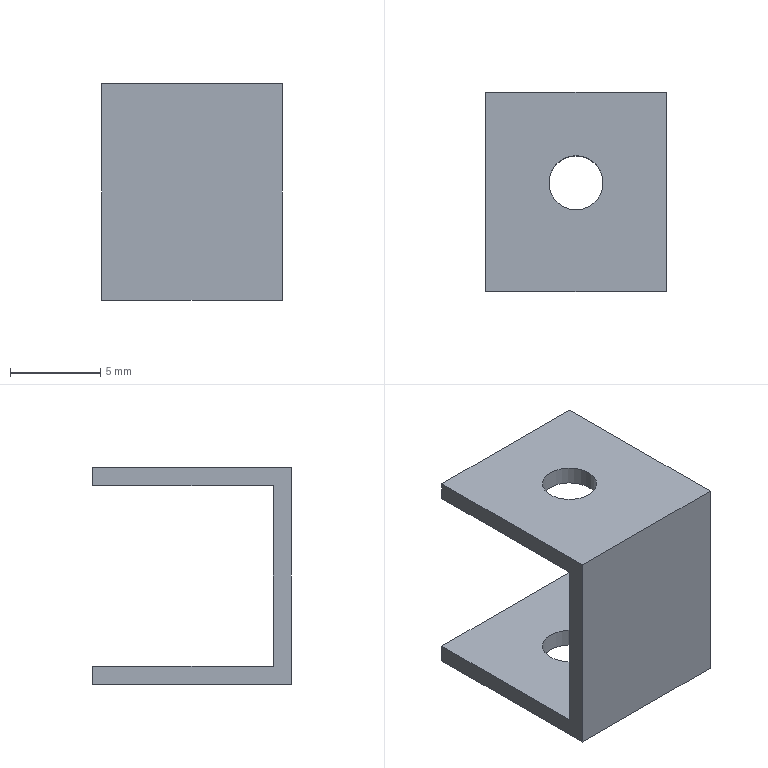Part | STEP file | 1-41.5 | 1 solid | 12 faces | box 10 x 11 x 12 mm | volume 305.863 mm3 | plane 10 | cylinder 2 | commonest cylinder face diameters 3 x2
STEP:
#1=CARTESIAN_POINT('',(0.,0.,0.));
#2=DIRECTION('',(0.,0.,1.));
#3=DIRECTION('',(1.,0.,0.));
#4=AXIS2_PLACEMENT_3D('',#1,#2,#3);
#5=CARTESIAN_POINT('',(5.,-5.5,-6.));
#6=VERTEX_POINT('',#5);
#7=CARTESIAN_POINT('',(5.,5.5,-6.));
#8=VERTEX_POINT('',#7);
#9=CARTESIAN_POINT('',(5.,-5.5,-6.));
#10=DIRECTION('',(0.,1.,0.));
#11=VECTOR('',#10,1.);
#12=LINE('',#9,#11);
#13=CARTESIAN_POINT('',(5.,0.5,0.));
#14=DIRECTION('',(1.,0.,0.));
#15=DIRECTION('',(0.,1.,0.));
#16=AXIS2_PLACEMENT_3D('',#13,#14,#15);
#17=PLANE('',#16);
#18=CARTESIAN_POINT('',(-6.,-6.));
#19=DIRECTION('',(1.,0.));
#20=VECTOR('',#19,1.);
#21=LINE('',#18,#20);
#22=(GEOMETRIC_REPRESENTATION_CONTEXT(2)PARAMETRIC_REPRESENTATION_CONTEXT()REPRESENTATION_CONTEXT('',''));
#23=DEFINITIONAL_REPRESENTATION('',(#21),#22);
#24=PCURVE('',#17,#23);
#25=CARTESIAN_POINT('',(0.,0.,-6.));
#26=DIRECTION('',(0.,0.,1.));
#27=DIRECTION('',(0.,1.,0.));
#28=AXIS2_PLACEMENT_3D('',#25,#26,#27);
#29=PLANE('',#28);
#30=CARTESIAN_POINT('',(-5.5,-5.));
#31=DIRECTION('',(1.,0.));
#32=VECTOR('',#31,1.);
#33=LINE('',#30,#32);
#34=(GEOMETRIC_REPRESENTATION_CONTEXT(2)PARAMETRIC_REPRESENTATION_CONTEXT()REPRESENTATION_CONTEXT('',''));
#35=DEFINITIONAL_REPRESENTATION('',(#33),#34);
#36=PCURVE('',#29,#35);
#37=SURFACE_CURVE('',#12,(#24,#36),.PCURVE_S1.);
#38=EDGE_CURVE('',#6,#8,#37,.T.);
#39=ORIENTED_EDGE('',*,*,#38,.T.);
#40=CARTESIAN_POINT('',(5.,5.5,-5.));
#41=VERTEX_POINT('',#40);
#42=CARTESIAN_POINT('',(5.,5.5,-6.));
#43=DIRECTION('',(0.,0.,1.));
#44=VECTOR('',#43,1.);
#45=LINE('',#42,#44);
#46=CARTESIAN_POINT('',(5.,-6.));
#47=DIRECTION('',(0.,1.));
#48=VECTOR('',#47,1.);
#49=LINE('',#46,#48);
#50=(GEOMETRIC_REPRESENTATION_CONTEXT(2)PARAMETRIC_REPRESENTATION_CONTEXT()REPRESENTATION_CONTEXT('',''));
#51=DEFINITIONAL_REPRESENTATION('',(#49),#50);
#52=PCURVE('',#17,#51);
#53=CARTESIAN_POINT('',(0.,5.5,-5.5));
#54=DIRECTION('',(0.,-1.,0.));
#55=DIRECTION('',(0.,0.,1.));
#56=AXIS2_PLACEMENT_3D('',#53,#54,#55);
#57=PLANE('',#56);
#58=CARTESIAN_POINT('',(-0.5,-5.));
#59=DIRECTION('',(1.,0.));
#60=VECTOR('',#59,1.);
#61=LINE('',#58,#60);
#62=(GEOMETRIC_REPRESENTATION_CONTEXT(2)PARAMETRIC_REPRESENTATION_CONTEXT()REPRESENTATION_CONTEXT('',''));
#63=DEFINITIONAL_REPRESENTATION('',(#61),#62);
#64=PCURVE('',#57,#63);
#65=SURFACE_CURVE('',#45,(#52,#64),.PCURVE_S1.);
#66=EDGE_CURVE('',#8,#41,#65,.T.);
#67=ORIENTED_EDGE('',*,*,#66,.T.);
#68=CARTESIAN_POINT('',(5.,-4.5,-5.));
#69=VERTEX_POINT('',#68);
#70=CARTESIAN_POINT('',(5.,5.5,-5.));
#71=DIRECTION('',(0.,-1.,0.));
#72=VECTOR('',#71,1.);
#73=LINE('',#70,#72);
#74=CARTESIAN_POINT('',(5.,-5.));
#75=DIRECTION('',(-1.,0.));
#76=VECTOR('',#75,1.);
#77=LINE('',#74,#76);
#78=(GEOMETRIC_REPRESENTATION_CONTEXT(2)PARAMETRIC_REPRESENTATION_CONTEXT()REPRESENTATION_CONTEXT('',''));
#79=DEFINITIONAL_REPRESENTATION('',(#77),#78);
#80=PCURVE('',#17,#79);
#81=CARTESIAN_POINT('',(0.,0.5,-5.));
#82=DIRECTION('',(0.,0.,-1.));
#83=DIRECTION('',(0.,-1.,0.));
#84=AXIS2_PLACEMENT_3D('',#81,#82,#83);
#85=PLANE('',#84);
#86=CARTESIAN_POINT('',(-5.,-5.));
#87=DIRECTION('',(1.,0.));
#88=VECTOR('',#87,1.);
#89=LINE('',#86,#88);
#90=(GEOMETRIC_REPRESENTATION_CONTEXT(2)PARAMETRIC_REPRESENTATION_CONTEXT()REPRESENTATION_CONTEXT('',''));
#91=DEFINITIONAL_REPRESENTATION('',(#89),#90);
#92=PCURVE('',#85,#91);
#93=SURFACE_CURVE('',#73,(#80,#92),.PCURVE_S1.);
#94=EDGE_CURVE('',#41,#69,#93,.T.);
#95=ORIENTED_EDGE('',*,*,#94,.T.);
#96=CARTESIAN_POINT('',(5.,-4.5,5.));
#97=VERTEX_POINT('',#96);
#98=CARTESIAN_POINT('',(5.,-4.5,-5.));
#99=DIRECTION('',(0.,0.,1.));
#100=VECTOR('',#99,1.);
#101=LINE('',#98,#100);
#102=CARTESIAN_POINT('',(-5.,-5.));
#103=DIRECTION('',(0.,1.));
#104=VECTOR('',#103,1.);
#105=LINE('',#102,#104);
#106=(GEOMETRIC_REPRESENTATION_CONTEXT(2)PARAMETRIC_REPRESENTATION_CONTEXT()REPRESENTATION_CONTEXT('',''));
#107=DEFINITIONAL_REPRESENTATION('',(#105),#106);
#108=PCURVE('',#17,#107);
#109=CARTESIAN_POINT('',(0.,-4.5,0.));
#110=DIRECTION('',(0.,-1.,0.));
#111=DIRECTION('',(0.,0.,1.));
#112=AXIS2_PLACEMENT_3D('',#109,#110,#111);
#113=PLANE('',#112);
#114=CARTESIAN_POINT('',(-5.,-5.));
#115=DIRECTION('',(1.,0.));
#116=VECTOR('',#115,1.);
#117=LINE('',#114,#116);
#118=(GEOMETRIC_REPRESENTATION_CONTEXT(2)PARAMETRIC_REPRESENTATION_CONTEXT()REPRESENTATION_CONTEXT('',''));
#119=DEFINITIONAL_REPRESENTATION('',(#117),#118);
#120=PCURVE('',#113,#119);
#121=SURFACE_CURVE('',#101,(#108,#120),.PCURVE_S1.);
#122=EDGE_CURVE('',#69,#97,#121,.T.);
#123=ORIENTED_EDGE('',*,*,#122,.T.);
#124=CARTESIAN_POINT('',(5.,5.5,5.));
#125=VERTEX_POINT('',#124);
#126=CARTESIAN_POINT('',(5.,-4.5,5.));
#127=DIRECTION('',(0.,1.,0.));
#128=VECTOR('',#127,1.);
#129=LINE('',#126,#128);
#130=CARTESIAN_POINT('',(-5.,5.));
#131=DIRECTION('',(1.,0.));
#132=VECTOR('',#131,1.);
#133=LINE('',#130,#132);
#134=(GEOMETRIC_REPRESENTATION_CONTEXT(2)PARAMETRIC_REPRESENTATION_CONTEXT()REPRESENTATION_CONTEXT('',''));
#135=DEFINITIONAL_REPRESENTATION('',(#133),#134);
#136=PCURVE('',#17,#135);
#137=CARTESIAN_POINT('',(0.,0.5,5.));
#138=DIRECTION('',(0.,0.,1.));
#139=DIRECTION('',(0.,1.,0.));
#140=AXIS2_PLACEMENT_3D('',#137,#138,#139);
#141=PLANE('',#140);
#142=CARTESIAN_POINT('',(-5.,-5.));
#143=DIRECTION('',(1.,0.));
#144=VECTOR('',#143,1.);
#145=LINE('',#142,#144);
#146=(GEOMETRIC_REPRESENTATION_CONTEXT(2)PARAMETRIC_REPRESENTATION_CONTEXT()REPRESENTATION_CONTEXT('',''));
#147=DEFINITIONAL_REPRESENTATION('',(#145),#146);
#148=PCURVE('',#141,#147);
#149=SURFACE_CURVE('',#129,(#136,#148),.PCURVE_S1.);
#150=EDGE_CURVE('',#97,#125,#149,.T.);
#151=ORIENTED_EDGE('',*,*,#150,.T.);
#152=CARTESIAN_POINT('',(5.,5.5,6.));
#153=VERTEX_POINT('',#152);
#154=CARTESIAN_POINT('',(5.,5.5,5.));
#155=DIRECTION('',(0.,0.,1.));
#156=VECTOR('',#155,1.);
#157=LINE('',#154,#156);
#158=CARTESIAN_POINT('',(5.,5.));
#159=DIRECTION('',(0.,1.));
#160=VECTOR('',#159,1.);
#161=LINE('',#158,#160);
#162=(GEOMETRIC_REPRESENTATION_CONTEXT(2)PARAMETRIC_REPRESENTATION_CONTEXT()REPRESENTATION_CONTEXT('',''));
#163=DEFINITIONAL_REPRESENTATION('',(#161),#162);
#164=PCURVE('',#17,#163);
#165=CARTESIAN_POINT('',(0.,5.5,5.5));
#166=DIRECTION('',(0.,-1.,0.));
#167=DIRECTION('',(0.,0.,1.));
#168=AXIS2_PLACEMENT_3D('',#165,#166,#167);
#169=PLANE('',#168);
#170=CARTESIAN_POINT('',(-0.5,-5.));
#171=DIRECTION('',(1.,0.));
#172=VECTOR('',#171,1.);
#173=LINE('',#170,#172);
#174=(GEOMETRIC_REPRESENTATION_CONTEXT(2)PARAMETRIC_REPRESENTATION_CONTEXT()REPRESENTATION_CONTEXT('',''));
#175=DEFINITIONAL_REPRESENTATION('',(#173),#174);
#176=PCURVE('',#169,#175);
#177=SURFACE_CURVE('',#157,(#164,#176),.PCURVE_S1.);
#178=EDGE_CURVE('',#125,#153,#177,.T.);
#179=ORIENTED_EDGE('',*,*,#178,.T.);
#180=CARTESIAN_POINT('',(5.,-5.5,6.));
#181=VERTEX_POINT('',#180);
#182=CARTESIAN_POINT('',(5.,5.5,6.));
#183=DIRECTION('',(0.,-1.,0.));
#184=VECTOR('',#183,1.);
#185=LINE('',#182,#184);
#186=CARTESIAN_POINT('',(5.,6.));
#187=DIRECTION('',(-1.,0.));
#188=VECTOR('',#187,1.);
#189=LINE('',#186,#188);
#190=(GEOMETRIC_REPRESENTATION_CONTEXT(2)PARAMETRIC_REPRESENTATION_CONTEXT()REPRESENTATION_CONTEXT('',''));
#191=DEFINITIONAL_REPRESENTATION('',(#189),#190);
#192=PCURVE('',#17,#191);
#193=CARTESIAN_POINT('',(0.,0.,6.));
#194=DIRECTION('',(0.,0.,-1.));
#195=DIRECTION('',(0.,-1.,0.));
#196=AXIS2_PLACEMENT_3D('',#193,#194,#195);
#197=PLANE('',#196);
#198=CARTESIAN_POINT('',(-5.5,-5.));
#199=DIRECTION('',(1.,0.));
#200=VECTOR('',#199,1.);
#201=LINE('',#198,#200);
#202=(GEOMETRIC_REPRESENTATION_CONTEXT(2)PARAMETRIC_REPRESENTATION_CONTEXT()REPRESENTATION_CONTEXT('',''));
#203=DEFINITIONAL_REPRESENTATION('',(#201),#202);
#204=PCURVE('',#197,#203);
#205=SURFACE_CURVE('',#185,(#192,#204),.PCURVE_S1.);
#206=EDGE_CURVE('',#153,#181,#205,.T.);
#207=ORIENTED_EDGE('',*,*,#206,.T.);
#208=CARTESIAN_POINT('',(5.,-5.5,6.));
#209=DIRECTION('',(0.,0.,-1.));
#210=VECTOR('',#209,1.);
#211=LINE('',#208,#210);
#212=CARTESIAN_POINT('',(-6.,6.));
#213=DIRECTION('',(0.,-1.));
#214=VECTOR('',#213,1.);
#215=LINE('',#212,#214);
#216=(GEOMETRIC_REPRESENTATION_CONTEXT(2)PARAMETRIC_REPRESENTATION_CONTEXT()REPRESENTATION_CONTEXT('',''));
#217=DEFINITIONAL_REPRESENTATION('',(#215),#216);
#218=PCURVE('',#17,#217);
#219=CARTESIAN_POINT('',(0.,-5.5,0.));
#220=DIRECTION('',(0.,1.,0.));
#221=DIRECTION('',(0.,0.,-1.));
#222=AXIS2_PLACEMENT_3D('',#219,#220,#221);
#223=PLANE('',#222);
#224=CARTESIAN_POINT('',(-6.,-5.));
#225=DIRECTION('',(1.,0.));
#226=VECTOR('',#225,1.);
#227=LINE('',#224,#226);
#228=(GEOMETRIC_REPRESENTATION_CONTEXT(2)PARAMETRIC_REPRESENTATION_CONTEXT()REPRESENTATION_CONTEXT('',''));
#229=DEFINITIONAL_REPRESENTATION('',(#227),#228);
#230=PCURVE('',#223,#229);
#231=SURFACE_CURVE('',#211,(#218,#230),.PCURVE_S1.);
#232=EDGE_CURVE('',#181,#6,#231,.T.);
#233=ORIENTED_EDGE('',*,*,#232,.T.);
#234=EDGE_LOOP('',(#39,#67,#95,#123,#151,#179,#207,#233));
#235=FACE_BOUND('',#234,.T.);
#236=ADVANCED_FACE('',(#235),#17,.T.);
#237=CARTESIAN_POINT('',(-5.,-5.5,-6.));
#238=VERTEX_POINT('',#237);
#239=CARTESIAN_POINT('',(-5.,5.5,-6.));
#240=VERTEX_POINT('',#239);
#241=CARTESIAN_POINT('',(-5.,-5.5,-6.));
#242=DIRECTION('',(0.,1.,0.));
#243=VECTOR('',#242,1.);
#244=LINE('',#241,#243);
#245=CARTESIAN_POINT('',(-5.,0.5,0.));
#246=DIRECTION('',(1.,0.,0.));
#247=DIRECTION('',(0.,1.,0.));
#248=AXIS2_PLACEMENT_3D('',#245,#246,#247);
#249=PLANE('',#248);
#250=CARTESIAN_POINT('',(-6.,-6.));
#251=DIRECTION('',(1.,0.));
#252=VECTOR('',#251,1.);
#253=LINE('',#250,#252);
#254=(GEOMETRIC_REPRESENTATION_CONTEXT(2)PARAMETRIC_REPRESENTATION_CONTEXT()REPRESENTATION_CONTEXT('',''));
#255=DEFINITIONAL_REPRESENTATION('',(#253),#254);
#256=PCURVE('',#249,#255);
#257=CARTESIAN_POINT('',(-5.5,5.));
#258=DIRECTION('',(1.,0.));
#259=VECTOR('',#258,1.);
#260=LINE('',#257,#259);
#261=(GEOMETRIC_REPRESENTATION_CONTEXT(2)PARAMETRIC_REPRESENTATION_CONTEXT()REPRESENTATION_CONTEXT('',''));
#262=DEFINITIONAL_REPRESENTATION('',(#260),#261);
#263=PCURVE('',#29,#262);
#264=SURFACE_CURVE('',#244,(#256,#263),.PCURVE_S1.);
#265=EDGE_CURVE('',#238,#240,#264,.T.);
#266=ORIENTED_EDGE('',*,*,#265,.T.);
#267=CARTESIAN_POINT('',(-5.,5.5,-5.));
#268=VERTEX_POINT('',#267);
#269=CARTESIAN_POINT('',(-5.,5.5,-6.));
#270=DIRECTION('',(0.,0.,1.));
#271=VECTOR('',#270,1.);
#272=LINE('',#269,#271);
#273=CARTESIAN_POINT('',(5.,-6.));
#274=DIRECTION('',(0.,1.));
#275=VECTOR('',#274,1.);
#276=LINE('',#273,#275);
#277=(GEOMETRIC_REPRESENTATION_CONTEXT(2)PARAMETRIC_REPRESENTATION_CONTEXT()REPRESENTATION_CONTEXT('',''));
#278=DEFINITIONAL_REPRESENTATION('',(#276),#277);
#279=PCURVE('',#249,#278);
#280=CARTESIAN_POINT('',(-0.5,5.));
#281=DIRECTION('',(1.,0.));
#282=VECTOR('',#281,1.);
#283=LINE('',#280,#282);
#284=(GEOMETRIC_REPRESENTATION_CONTEXT(2)PARAMETRIC_REPRESENTATION_CONTEXT()REPRESENTATION_CONTEXT('',''));
#285=DEFINITIONAL_REPRESENTATION('',(#283),#284);
#286=PCURVE('',#57,#285);
#287=SURFACE_CURVE('',#272,(#279,#286),.PCURVE_S1.);
#288=EDGE_CURVE('',#240,#268,#287,.T.);
#289=ORIENTED_EDGE('',*,*,#288,.T.);
#290=CARTESIAN_POINT('',(-5.,-4.5,-5.));
#291=VERTEX_POINT('',#290);
#292=CARTESIAN_POINT('',(-5.,5.5,-5.));
#293=DIRECTION('',(0.,-1.,0.));
#294=VECTOR('',#293,1.);
#295=LINE('',#292,#294);
#296=CARTESIAN_POINT('',(5.,-5.));
#297=DIRECTION('',(-1.,0.));
#298=VECTOR('',#297,1.);
#299=LINE('',#296,#298);
#300=(GEOMETRIC_REPRESENTATION_CONTEXT(2)PARAMETRIC_REPRESENTATION_CONTEXT()REPRESENTATION_CONTEXT('',''));
#301=DEFINITIONAL_REPRESENTATION('',(#299),#300);
#302=PCURVE('',#249,#301);
#303=CARTESIAN_POINT('',(-5.,5.));
#304=DIRECTION('',(1.,0.));
#305=VECTOR('',#304,1.);
#306=LINE('',#303,#305);
#307=(GEOMETRIC_REPRESENTATION_CONTEXT(2)PARAMETRIC_REPRESENTATION_CONTEXT()REPRESENTATION_CONTEXT('',''));
#308=DEFINITIONAL_REPRESENTATION('',(#306),#307);
#309=PCURVE('',#85,#308);
#310=SURFACE_CURVE('',#295,(#302,#309),.PCURVE_S1.);
#311=EDGE_CURVE('',#268,#291,#310,.T.);
#312=ORIENTED_EDGE('',*,*,#311,.T.);
#313=CARTESIAN_POINT('',(-5.,-4.5,5.));
#314=VERTEX_POINT('',#313);
#315=CARTESIAN_POINT('',(-5.,-4.5,-5.));
#316=DIRECTION('',(0.,0.,1.));
#317=VECTOR('',#316,1.);
#318=LINE('',#315,#317);
#319=CARTESIAN_POINT('',(-5.,-5.));
#320=DIRECTION('',(0.,1.));
#321=VECTOR('',#320,1.);
#322=LINE('',#319,#321);
#323=(GEOMETRIC_REPRESENTATION_CONTEXT(2)PARAMETRIC_REPRESENTATION_CONTEXT()REPRESENTATION_CONTEXT('',''));
#324=DEFINITIONAL_REPRESENTATION('',(#322),#323);
#325=PCURVE('',#249,#324);
#326=CARTESIAN_POINT('',(-5.,5.));
#327=DIRECTION('',(1.,0.));
#328=VECTOR('',#327,1.);
#329=LINE('',#326,#328);
#330=(GEOMETRIC_REPRESENTATION_CONTEXT(2)PARAMETRIC_REPRESENTATION_CONTEXT()REPRESENTATION_CONTEXT('',''));
#331=DEFINITIONAL_REPRESENTATION('',(#329),#330);
#332=PCURVE('',#113,#331);
#333=SURFACE_CURVE('',#318,(#325,#332),.PCURVE_S1.);
#334=EDGE_CURVE('',#291,#314,#333,.T.);
#335=ORIENTED_EDGE('',*,*,#334,.T.);
#336=CARTESIAN_POINT('',(-5.,5.5,5.));
#337=VERTEX_POINT('',#336);
#338=CARTESIAN_POINT('',(-5.,-4.5,5.));
#339=DIRECTION('',(0.,1.,0.));
#340=VECTOR('',#339,1.);
#341=LINE('',#338,#340);
#342=CARTESIAN_POINT('',(-5.,5.));
#343=DIRECTION('',(1.,0.));
#344=VECTOR('',#343,1.);
#345=LINE('',#342,#344);
#346=(GEOMETRIC_REPRESENTATION_CONTEXT(2)PARAMETRIC_REPRESENTATION_CONTEXT()REPRESENTATION_CONTEXT('',''));
#347=DEFINITIONAL_REPRESENTATION('',(#345),#346);
#348=PCURVE('',#249,#347);
#349=CARTESIAN_POINT('',(-5.,5.));
#350=DIRECTION('',(1.,0.));
#351=VECTOR('',#350,1.);
#352=LINE('',#349,#351);
#353=(GEOMETRIC_REPRESENTATION_CONTEXT(2)PARAMETRIC_REPRESENTATION_CONTEXT()REPRESENTATION_CONTEXT('',''));
#354=DEFINITIONAL_REPRESENTATION('',(#352),#353);
#355=PCURVE('',#141,#354);
#356=SURFACE_CURVE('',#341,(#348,#355),.PCURVE_S1.);
#357=EDGE_CURVE('',#314,#337,#356,.T.);
#358=ORIENTED_EDGE('',*,*,#357,.T.);
#359=CARTESIAN_POINT('',(-5.,5.5,6.));
#360=VERTEX_POINT('',#359);
#361=CARTESIAN_POINT('',(-5.,5.5,5.));
#362=DIRECTION('',(0.,0.,1.));
#363=VECTOR('',#362,1.);
#364=LINE('',#361,#363);
#365=CARTESIAN_POINT('',(5.,5.));
#366=DIRECTION('',(0.,1.));
#367=VECTOR('',#366,1.);
#368=LINE('',#365,#367);
#369=(GEOMETRIC_REPRESENTATION_CONTEXT(2)PARAMETRIC_REPRESENTATION_CONTEXT()REPRESENTATION_CONTEXT('',''));
#370=DEFINITIONAL_REPRESENTATION('',(#368),#369);
#371=PCURVE('',#249,#370);
#372=CARTESIAN_POINT('',(-0.5,5.));
#373=DIRECTION('',(1.,0.));
#374=VECTOR('',#373,1.);
#375=LINE('',#372,#374);
#376=(GEOMETRIC_REPRESENTATION_CONTEXT(2)PARAMETRIC_REPRESENTATION_CONTEXT()REPRESENTATION_CONTEXT('',''));
#377=DEFINITIONAL_REPRESENTATION('',(#375),#376);
#378=PCURVE('',#169,#377);
#379=SURFACE_CURVE('',#364,(#371,#378),.PCURVE_S1.);
#380=EDGE_CURVE('',#337,#360,#379,.T.);
#381=ORIENTED_EDGE('',*,*,#380,.T.);
#382=CARTESIAN_POINT('',(-5.,-5.5,6.));
#383=VERTEX_POINT('',#382);
#384=CARTESIAN_POINT('',(-5.,5.5,6.));
#385=DIRECTION('',(0.,-1.,0.));
#386=VECTOR('',#385,1.);
#387=LINE('',#384,#386);
#388=CARTESIAN_POINT('',(5.,6.));
#389=DIRECTION('',(-1.,0.));
#390=VECTOR('',#389,1.);
#391=LINE('',#388,#390);
#392=(GEOMETRIC_REPRESENTATION_CONTEXT(2)PARAMETRIC_REPRESENTATION_CONTEXT()REPRESENTATION_CONTEXT('',''));
#393=DEFINITIONAL_REPRESENTATION('',(#391),#392);
#394=PCURVE('',#249,#393);
#395=CARTESIAN_POINT('',(-5.5,5.));
#396=DIRECTION('',(1.,0.));
#397=VECTOR('',#396,1.);
#398=LINE('',#395,#397);
#399=(GEOMETRIC_REPRESENTATION_CONTEXT(2)PARAMETRIC_REPRESENTATION_CONTEXT()REPRESENTATION_CONTEXT('',''));
#400=DEFINITIONAL_REPRESENTATION('',(#398),#399);
#401=PCURVE('',#197,#400);
#402=SURFACE_CURVE('',#387,(#394,#401),.PCURVE_S1.);
#403=EDGE_CURVE('',#360,#383,#402,.T.);
#404=ORIENTED_EDGE('',*,*,#403,.T.);
#405=CARTESIAN_POINT('',(-5.,-5.5,6.));
#406=DIRECTION('',(0.,0.,-1.));
#407=VECTOR('',#406,1.);
#408=LINE('',#405,#407);
#409=CARTESIAN_POINT('',(-6.,6.));
#410=DIRECTION('',(0.,-1.));
#411=VECTOR('',#410,1.);
#412=LINE('',#409,#411);
#413=(GEOMETRIC_REPRESENTATION_CONTEXT(2)PARAMETRIC_REPRESENTATION_CONTEXT()REPRESENTATION_CONTEXT('',''));
#414=DEFINITIONAL_REPRESENTATION('',(#412),#413);
#415=PCURVE('',#249,#414);
#416=CARTESIAN_POINT('',(-6.,5.));
#417=DIRECTION('',(1.,0.));
#418=VECTOR('',#417,1.);
#419=LINE('',#416,#418);
#420=(GEOMETRIC_REPRESENTATION_CONTEXT(2)PARAMETRIC_REPRESENTATION_CONTEXT()REPRESENTATION_CONTEXT('',''));
#421=DEFINITIONAL_REPRESENTATION('',(#419),#420);
#422=PCURVE('',#223,#421);
#423=SURFACE_CURVE('',#408,(#415,#422),.PCURVE_S1.);
#424=EDGE_CURVE('',#383,#238,#423,.T.);
#425=ORIENTED_EDGE('',*,*,#424,.T.);
#426=EDGE_LOOP('',(#266,#289,#312,#335,#358,#381,#404,#425));
#427=FACE_BOUND('',#426,.F.);
#428=ADVANCED_FACE('',(#427),#249,.F.);
#429=ORIENTED_EDGE('',*,*,#66,.T.);
#430=CARTESIAN_POINT('',(5.,5.5,-5.));
#431=DIRECTION('',(-1.,0.,0.));
#432=VECTOR('',#431,1.);
#433=LINE('',#430,#432);
#434=CARTESIAN_POINT('',(0.5,-5.));
#435=DIRECTION('',(0.,1.));
#436=VECTOR('',#435,1.);
#437=LINE('',#434,#436);
#438=(GEOMETRIC_REPRESENTATION_CONTEXT(2)PARAMETRIC_REPRESENTATION_CONTEXT()REPRESENTATION_CONTEXT('',''));
#439=DEFINITIONAL_REPRESENTATION('',(#437),#438);
#440=PCURVE('',#57,#439);
#441=CARTESIAN_POINT('',(-5.,-5.));
#442=DIRECTION('',(0.,1.));
#443=VECTOR('',#442,1.);
#444=LINE('',#441,#443);
#445=(GEOMETRIC_REPRESENTATION_CONTEXT(2)PARAMETRIC_REPRESENTATION_CONTEXT()REPRESENTATION_CONTEXT('',''));
#446=DEFINITIONAL_REPRESENTATION('',(#444),#445);
#447=PCURVE('',#85,#446);
#448=SURFACE_CURVE('',#433,(#440,#447),.PCURVE_S1.);
#449=EDGE_CURVE('',#41,#268,#448,.T.);
#450=ORIENTED_EDGE('',*,*,#449,.T.);
#451=ORIENTED_EDGE('',*,*,#288,.F.);
#452=CARTESIAN_POINT('',(5.,5.5,-6.));
#453=DIRECTION('',(-1.,0.,0.));
#454=VECTOR('',#453,1.);
#455=LINE('',#452,#454);
#456=CARTESIAN_POINT('',(-0.5,-5.));
#457=DIRECTION('',(0.,1.));
#458=VECTOR('',#457,1.);
#459=LINE('',#456,#458);
#460=(GEOMETRIC_REPRESENTATION_CONTEXT(2)PARAMETRIC_REPRESENTATION_CONTEXT()REPRESENTATION_CONTEXT('',''));
#461=DEFINITIONAL_REPRESENTATION('',(#459),#460);
#462=PCURVE('',#57,#461);
#463=CARTESIAN_POINT('',(5.5,-5.));
#464=DIRECTION('',(0.,1.));
#465=VECTOR('',#464,1.);
#466=LINE('',#463,#465);
#467=(GEOMETRIC_REPRESENTATION_CONTEXT(2)PARAMETRIC_REPRESENTATION_CONTEXT()REPRESENTATION_CONTEXT('',''));
#468=DEFINITIONAL_REPRESENTATION('',(#466),#467);
#469=PCURVE('',#29,#468);
#470=SURFACE_CURVE('',#455,(#462,#469),.PCURVE_S1.);
#471=EDGE_CURVE('',#8,#240,#470,.T.);
#472=ORIENTED_EDGE('',*,*,#471,.F.);
#473=EDGE_LOOP('',(#429,#450,#451,#472));
#474=FACE_BOUND('',#473,.F.);
#475=ADVANCED_FACE('',(#474),#57,.F.);
#476=ORIENTED_EDGE('',*,*,#122,.T.);
#477=CARTESIAN_POINT('',(5.,-4.5,5.));
#478=DIRECTION('',(-1.,0.,0.));
#479=VECTOR('',#478,1.);
#480=LINE('',#477,#479);
#481=CARTESIAN_POINT('',(5.,-5.));
#482=DIRECTION('',(0.,1.));
#483=VECTOR('',#482,1.);
#484=LINE('',#481,#483);
#485=(GEOMETRIC_REPRESENTATION_CONTEXT(2)PARAMETRIC_REPRESENTATION_CONTEXT()REPRESENTATION_CONTEXT('',''));
#486=DEFINITIONAL_REPRESENTATION('',(#484),#485);
#487=PCURVE('',#113,#486);
#488=CARTESIAN_POINT('',(-5.,-5.));
#489=DIRECTION('',(0.,1.));
#490=VECTOR('',#489,1.);
#491=LINE('',#488,#490);
#492=(GEOMETRIC_REPRESENTATION_CONTEXT(2)PARAMETRIC_REPRESENTATION_CONTEXT()REPRESENTATION_CONTEXT('',''));
#493=DEFINITIONAL_REPRESENTATION('',(#491),#492);
#494=PCURVE('',#141,#493);
#495=SURFACE_CURVE('',#480,(#487,#494),.PCURVE_S1.);
#496=EDGE_CURVE('',#97,#314,#495,.T.);
#497=ORIENTED_EDGE('',*,*,#496,.T.);
#498=ORIENTED_EDGE('',*,*,#334,.F.);
#499=CARTESIAN_POINT('',(5.,-4.5,-5.));
#500=DIRECTION('',(-1.,0.,0.));
#501=VECTOR('',#500,1.);
#502=LINE('',#499,#501);
#503=CARTESIAN_POINT('',(-5.,-5.));
#504=DIRECTION('',(0.,1.));
#505=VECTOR('',#504,1.);
#506=LINE('',#503,#505);
#507=(GEOMETRIC_REPRESENTATION_CONTEXT(2)PARAMETRIC_REPRESENTATION_CONTEXT()REPRESENTATION_CONTEXT('',''));
#508=DEFINITIONAL_REPRESENTATION('',(#506),#507);
#509=PCURVE('',#113,#508);
#510=CARTESIAN_POINT('',(5.,-5.));
#511=DIRECTION('',(0.,1.));
#512=VECTOR('',#511,1.);
#513=LINE('',#510,#512);
#514=(GEOMETRIC_REPRESENTATION_CONTEXT(2)PARAMETRIC_REPRESENTATION_CONTEXT()REPRESENTATION_CONTEXT('',''));
#515=DEFINITIONAL_REPRESENTATION('',(#513),#514);
#516=PCURVE('',#85,#515);
#517=SURFACE_CURVE('',#502,(#509,#516),.PCURVE_S1.);
#518=EDGE_CURVE('',#69,#291,#517,.T.);
#519=ORIENTED_EDGE('',*,*,#518,.F.);
#520=EDGE_LOOP('',(#476,#497,#498,#519));
#521=FACE_BOUND('',#520,.F.);
#522=ADVANCED_FACE('',(#521),#113,.F.);
#523=ORIENTED_EDGE('',*,*,#178,.T.);
#524=CARTESIAN_POINT('',(5.,5.5,6.));
#525=DIRECTION('',(-1.,0.,0.));
#526=VECTOR('',#525,1.);
#527=LINE('',#524,#526);
#528=CARTESIAN_POINT('',(0.5,-5.));
#529=DIRECTION('',(0.,1.));
#530=VECTOR('',#529,1.);
#531=LINE('',#528,#530);
#532=(GEOMETRIC_REPRESENTATION_CONTEXT(2)PARAMETRIC_REPRESENTATION_CONTEXT()REPRESENTATION_CONTEXT('',''));
#533=DEFINITIONAL_REPRESENTATION('',(#531),#532);
#534=PCURVE('',#169,#533);
#535=CARTESIAN_POINT('',(-5.5,-5.));
#536=DIRECTION('',(0.,1.));
#537=VECTOR('',#536,1.);
#538=LINE('',#535,#537);
#539=(GEOMETRIC_REPRESENTATION_CONTEXT(2)PARAMETRIC_REPRESENTATION_CONTEXT()REPRESENTATION_CONTEXT('',''));
#540=DEFINITIONAL_REPRESENTATION('',(#538),#539);
#541=PCURVE('',#197,#540);
#542=SURFACE_CURVE('',#527,(#534,#541),.PCURVE_S1.);
#543=EDGE_CURVE('',#153,#360,#542,.T.);
#544=ORIENTED_EDGE('',*,*,#543,.T.);
#545=ORIENTED_EDGE('',*,*,#380,.F.);
#546=CARTESIAN_POINT('',(5.,5.5,5.));
#547=DIRECTION('',(-1.,0.,0.));
#548=VECTOR('',#547,1.);
#549=LINE('',#546,#548);
#550=CARTESIAN_POINT('',(-0.5,-5.));
#551=DIRECTION('',(0.,1.));
#552=VECTOR('',#551,1.);
#553=LINE('',#550,#552);
#554=(GEOMETRIC_REPRESENTATION_CONTEXT(2)PARAMETRIC_REPRESENTATION_CONTEXT()REPRESENTATION_CONTEXT('',''));
#555=DEFINITIONAL_REPRESENTATION('',(#553),#554);
#556=PCURVE('',#169,#555);
#557=CARTESIAN_POINT('',(5.,-5.));
#558=DIRECTION('',(0.,1.));
#559=VECTOR('',#558,1.);
#560=LINE('',#557,#559);
#561=(GEOMETRIC_REPRESENTATION_CONTEXT(2)PARAMETRIC_REPRESENTATION_CONTEXT()REPRESENTATION_CONTEXT('',''));
#562=DEFINITIONAL_REPRESENTATION('',(#560),#561);
#563=PCURVE('',#141,#562);
#564=SURFACE_CURVE('',#549,(#556,#563),.PCURVE_S1.);
#565=EDGE_CURVE('',#125,#337,#564,.T.);
#566=ORIENTED_EDGE('',*,*,#565,.F.);
#567=EDGE_LOOP('',(#523,#544,#545,#566));
#568=FACE_BOUND('',#567,.F.);
#569=ADVANCED_FACE('',(#568),#169,.F.);
#570=ORIENTED_EDGE('',*,*,#232,.T.);
#571=CARTESIAN_POINT('',(5.,-5.5,-6.));
#572=DIRECTION('',(-1.,0.,0.));
#573=VECTOR('',#572,1.);
#574=LINE('',#571,#573);
#575=CARTESIAN_POINT('',(6.,-5.));
#576=DIRECTION('',(0.,1.));
#577=VECTOR('',#576,1.);
#578=LINE('',#575,#577);
#579=(GEOMETRIC_REPRESENTATION_CONTEXT(2)PARAMETRIC_REPRESENTATION_CONTEXT()REPRESENTATION_CONTEXT('',''));
#580=DEFINITIONAL_REPRESENTATION('',(#578),#579);
#581=PCURVE('',#223,#580);
#582=CARTESIAN_POINT('',(-5.5,-5.));
#583=DIRECTION('',(0.,1.));
#584=VECTOR('',#583,1.);
#585=LINE('',#582,#584);
#586=(GEOMETRIC_REPRESENTATION_CONTEXT(2)PARAMETRIC_REPRESENTATION_CONTEXT()REPRESENTATION_CONTEXT('',''));
#587=DEFINITIONAL_REPRESENTATION('',(#585),#586);
#588=PCURVE('',#29,#587);
#589=SURFACE_CURVE('',#574,(#581,#588),.PCURVE_S1.);
#590=EDGE_CURVE('',#6,#238,#589,.T.);
#591=ORIENTED_EDGE('',*,*,#590,.T.);
#592=ORIENTED_EDGE('',*,*,#424,.F.);
#593=CARTESIAN_POINT('',(5.,-5.5,6.));
#594=DIRECTION('',(-1.,0.,0.));
#595=VECTOR('',#594,1.);
#596=LINE('',#593,#595);
#597=CARTESIAN_POINT('',(-6.,-5.));
#598=DIRECTION('',(0.,1.));
#599=VECTOR('',#598,1.);
#600=LINE('',#597,#599);
#601=(GEOMETRIC_REPRESENTATION_CONTEXT(2)PARAMETRIC_REPRESENTATION_CONTEXT()REPRESENTATION_CONTEXT('',''));
#602=DEFINITIONAL_REPRESENTATION('',(#600),#601);
#603=PCURVE('',#223,#602);
#604=CARTESIAN_POINT('',(5.5,-5.));
#605=DIRECTION('',(0.,1.));
#606=VECTOR('',#605,1.);
#607=LINE('',#604,#606);
#608=(GEOMETRIC_REPRESENTATION_CONTEXT(2)PARAMETRIC_REPRESENTATION_CONTEXT()REPRESENTATION_CONTEXT('',''));
#609=DEFINITIONAL_REPRESENTATION('',(#607),#608);
#610=PCURVE('',#197,#609);
#611=SURFACE_CURVE('',#596,(#603,#610),.PCURVE_S1.);
#612=EDGE_CURVE('',#181,#383,#611,.T.);
#613=ORIENTED_EDGE('',*,*,#612,.F.);
#614=EDGE_LOOP('',(#570,#591,#592,#613));
#615=FACE_BOUND('',#614,.F.);
#616=ADVANCED_FACE('',(#615),#223,.F.);
#617=ORIENTED_EDGE('',*,*,#38,.T.);
#618=ORIENTED_EDGE('',*,*,#471,.T.);
#619=ORIENTED_EDGE('',*,*,#265,.F.);
#620=ORIENTED_EDGE('',*,*,#590,.F.);
#621=EDGE_LOOP('',(#617,#618,#619,#620));
#622=FACE_BOUND('',#621,.F.);
#623=CARTESIAN_POINT('',(0.,2.,-6.));
#624=VERTEX_POINT('',#623);
#625=CARTESIAN_POINT('',(0.,0.5,-6.));
#626=DIRECTION('',(0.,0.,-1.));
#627=DIRECTION('',(0.,1.,0.));
#628=AXIS2_PLACEMENT_3D('',#625,#626,#627);
#629=CIRCLE('',#628,1.5);
#630=CARTESIAN_POINT('',(2.,0.));
#631=CARTESIAN_POINT('',(2.,-2.598));
#632=CARTESIAN_POINT('',(-0.25,-1.299));
#633=CARTESIAN_POINT('',(-2.5,0.));
#634=CARTESIAN_POINT('',(-0.25,1.299));
#635=CARTESIAN_POINT('',(2.,2.598));
#636=CARTESIAN_POINT('',(2.,0.));
#637=(BOUNDED_CURVE()B_SPLINE_CURVE(2,(#630,#631,#632,#633,#634,#635,#636),.UNSPECIFIED.,.T.,.F.)B_SPLINE_CURVE_WITH_KNOTS((1,2,2,2,2,1),(-2.094,0.,2.094,4.189,6.283,8.378),.UNSPECIFIED.)CURVE()GEOMETRIC_REPRESENTATION_ITEM()RATIONAL_B_SPLINE_CURVE((1.,0.5,1.,0.5,1.,0.5,1.))REPRESENTATION_ITEM(''));
#638=(GEOMETRIC_REPRESENTATION_CONTEXT(2)PARAMETRIC_REPRESENTATION_CONTEXT()REPRESENTATION_CONTEXT('',''));
#639=DEFINITIONAL_REPRESENTATION('',(#637),#638);
#640=PCURVE('',#29,#639);
#641=CARTESIAN_POINT('',(0.,0.5,6.5));
#642=DIRECTION('',(0.,0.,-1.));
#643=DIRECTION('',(0.,1.,0.));
#644=AXIS2_PLACEMENT_3D('',#641,#642,#643);
#645=CYLINDRICAL_SURFACE('',#644,1.5);
#646=CARTESIAN_POINT('',(0.,12.5));
#647=DIRECTION('',(1.,0.));
#648=VECTOR('',#647,1.);
#649=LINE('',#646,#648);
#650=(GEOMETRIC_REPRESENTATION_CONTEXT(2)PARAMETRIC_REPRESENTATION_CONTEXT()REPRESENTATION_CONTEXT('',''));
#651=DEFINITIONAL_REPRESENTATION('',(#649),#650);
#652=PCURVE('',#645,#651);
#653=SURFACE_CURVE('',#629,(#640,#652),.PCURVE_S1.);
#654=EDGE_CURVE('',#624,#624,#653,.T.);
#655=ORIENTED_EDGE('',*,*,#654,.T.);
#656=EDGE_LOOP('',(#655));
#657=FACE_BOUND('',#656,.F.);
#658=ADVANCED_FACE('',(#622,#657),#29,.F.);
#659=ORIENTED_EDGE('',*,*,#94,.T.);
#660=ORIENTED_EDGE('',*,*,#518,.T.);
#661=ORIENTED_EDGE('',*,*,#311,.F.);
#662=ORIENTED_EDGE('',*,*,#449,.F.);
#663=EDGE_LOOP('',(#659,#660,#661,#662));
#664=FACE_BOUND('',#663,.F.);
#665=CARTESIAN_POINT('',(0.,2.,-5.));
#666=VERTEX_POINT('',#665);
#667=CARTESIAN_POINT('',(0.,0.5,-5.));
#668=DIRECTION('',(0.,0.,1.));
#669=DIRECTION('',(0.,1.,0.));
#670=AXIS2_PLACEMENT_3D('',#667,#668,#669);
#671=CIRCLE('',#670,1.5);
#672=CARTESIAN_POINT('',(-1.5,0.));
#673=CARTESIAN_POINT('',(-1.5,2.598));
#674=CARTESIAN_POINT('',(0.75,1.299));
#675=CARTESIAN_POINT('',(3.,0.));
#676=CARTESIAN_POINT('',(0.75,-1.299));
#677=CARTESIAN_POINT('',(-1.5,-2.598));
#678=CARTESIAN_POINT('',(-1.5,0.));
#679=(BOUNDED_CURVE()B_SPLINE_CURVE(2,(#672,#673,#674,#675,#676,#677,#678),.UNSPECIFIED.,.T.,.F.)B_SPLINE_CURVE_WITH_KNOTS((1,2,2,2,2,1),(-2.094,0.,2.094,4.189,6.283,8.378),.UNSPECIFIED.)CURVE()GEOMETRIC_REPRESENTATION_ITEM()RATIONAL_B_SPLINE_CURVE((1.,0.5,1.,0.5,1.,0.5,1.))REPRESENTATION_ITEM(''));
#680=(GEOMETRIC_REPRESENTATION_CONTEXT(2)PARAMETRIC_REPRESENTATION_CONTEXT()REPRESENTATION_CONTEXT('',''));
#681=DEFINITIONAL_REPRESENTATION('',(#679),#680);
#682=PCURVE('',#85,#681);
#683=CARTESIAN_POINT('',(6.283,11.5));
#684=DIRECTION('',(-1.,0.));
#685=VECTOR('',#684,1.);
#686=LINE('',#683,#685);
#687=(GEOMETRIC_REPRESENTATION_CONTEXT(2)PARAMETRIC_REPRESENTATION_CONTEXT()REPRESENTATION_CONTEXT('',''));
#688=DEFINITIONAL_REPRESENTATION('',(#686),#687);
#689=PCURVE('',#645,#688);
#690=SURFACE_CURVE('',#671,(#682,#689),.PCURVE_S1.);
#691=EDGE_CURVE('',#666,#666,#690,.T.);
#692=ORIENTED_EDGE('',*,*,#691,.T.);
#693=EDGE_LOOP('',(#692));
#694=FACE_BOUND('',#693,.F.);
#695=ADVANCED_FACE('',(#664,#694),#85,.F.);
#696=ORIENTED_EDGE('',*,*,#150,.T.);
#697=ORIENTED_EDGE('',*,*,#565,.T.);
#698=ORIENTED_EDGE('',*,*,#357,.F.);
#699=ORIENTED_EDGE('',*,*,#496,.F.);
#700=EDGE_LOOP('',(#696,#697,#698,#699));
#701=FACE_BOUND('',#700,.F.);
#702=CARTESIAN_POINT('',(0.,2.,5.));
#703=VERTEX_POINT('',#702);
#704=CARTESIAN_POINT('',(0.,0.5,5.));
#705=DIRECTION('',(0.,0.,-1.));
#706=DIRECTION('',(0.,1.,0.));
#707=AXIS2_PLACEMENT_3D('',#704,#705,#706);
#708=CIRCLE('',#707,1.5);
#709=CARTESIAN_POINT('',(1.5,0.));
#710=CARTESIAN_POINT('',(1.5,-2.598));
#711=CARTESIAN_POINT('',(-0.75,-1.299));
#712=CARTESIAN_POINT('',(-3.,0.));
#713=CARTESIAN_POINT('',(-0.75,1.299));
#714=CARTESIAN_POINT('',(1.5,2.598));
#715=CARTESIAN_POINT('',(1.5,0.));
#716=(BOUNDED_CURVE()B_SPLINE_CURVE(2,(#709,#710,#711,#712,#713,#714,#715),.UNSPECIFIED.,.T.,.F.)B_SPLINE_CURVE_WITH_KNOTS((1,2,2,2,2,1),(-2.094,0.,2.094,4.189,6.283,8.378),.UNSPECIFIED.)CURVE()GEOMETRIC_REPRESENTATION_ITEM()RATIONAL_B_SPLINE_CURVE((1.,0.5,1.,0.5,1.,0.5,1.))REPRESENTATION_ITEM(''));
#717=(GEOMETRIC_REPRESENTATION_CONTEXT(2)PARAMETRIC_REPRESENTATION_CONTEXT()REPRESENTATION_CONTEXT('',''));
#718=DEFINITIONAL_REPRESENTATION('',(#716),#717);
#719=PCURVE('',#141,#718);
#720=CARTESIAN_POINT('',(0.,0.5,6.5));
#721=DIRECTION('',(0.,0.,-1.));
#722=DIRECTION('',(0.,1.,0.));
#723=AXIS2_PLACEMENT_3D('',#720,#721,#722);
#724=CYLINDRICAL_SURFACE('',#723,1.5);
#725=CARTESIAN_POINT('',(0.,1.5));
#726=DIRECTION('',(1.,0.));
#727=VECTOR('',#726,1.);
#728=LINE('',#725,#727);
#729=(GEOMETRIC_REPRESENTATION_CONTEXT(2)PARAMETRIC_REPRESENTATION_CONTEXT()REPRESENTATION_CONTEXT('',''));
#730=DEFINITIONAL_REPRESENTATION('',(#728),#729);
#731=PCURVE('',#724,#730);
#732=SURFACE_CURVE('',#708,(#719,#731),.PCURVE_S1.);
#733=EDGE_CURVE('',#703,#703,#732,.T.);
#734=ORIENTED_EDGE('',*,*,#733,.T.);
#735=EDGE_LOOP('',(#734));
#736=FACE_BOUND('',#735,.F.);
#737=ADVANCED_FACE('',(#701,#736),#141,.F.);
#738=ORIENTED_EDGE('',*,*,#206,.T.);
#739=ORIENTED_EDGE('',*,*,#612,.T.);
#740=ORIENTED_EDGE('',*,*,#403,.F.);
#741=ORIENTED_EDGE('',*,*,#543,.F.);
#742=EDGE_LOOP('',(#738,#739,#740,#741));
#743=FACE_BOUND('',#742,.F.);
#744=CARTESIAN_POINT('',(0.,2.,6.));
#745=VERTEX_POINT('',#744);
#746=CARTESIAN_POINT('',(0.,0.5,6.));
#747=DIRECTION('',(0.,0.,1.));
#748=DIRECTION('',(0.,1.,0.));
#749=AXIS2_PLACEMENT_3D('',#746,#747,#748);
#750=CIRCLE('',#749,1.5);
#751=CARTESIAN_POINT('',(-2.,0.));
#752=CARTESIAN_POINT('',(-2.,2.598));
#753=CARTESIAN_POINT('',(0.25,1.299));
#754=CARTESIAN_POINT('',(2.5,0.));
#755=CARTESIAN_POINT('',(0.25,-1.299));
#756=CARTESIAN_POINT('',(-2.,-2.598));
#757=CARTESIAN_POINT('',(-2.,0.));
#758=(BOUNDED_CURVE()B_SPLINE_CURVE(2,(#751,#752,#753,#754,#755,#756,#757),.UNSPECIFIED.,.T.,.F.)B_SPLINE_CURVE_WITH_KNOTS((1,2,2,2,2,1),(-2.094,0.,2.094,4.189,6.283,8.378),.UNSPECIFIED.)CURVE()GEOMETRIC_REPRESENTATION_ITEM()RATIONAL_B_SPLINE_CURVE((1.,0.5,1.,0.5,1.,0.5,1.))REPRESENTATION_ITEM(''));
#759=(GEOMETRIC_REPRESENTATION_CONTEXT(2)PARAMETRIC_REPRESENTATION_CONTEXT()REPRESENTATION_CONTEXT('',''));
#760=DEFINITIONAL_REPRESENTATION('',(#758),#759);
#761=PCURVE('',#197,#760);
#762=CARTESIAN_POINT('',(6.283,0.5));
#763=DIRECTION('',(-1.,0.));
#764=VECTOR('',#763,1.);
#765=LINE('',#762,#764);
#766=(GEOMETRIC_REPRESENTATION_CONTEXT(2)PARAMETRIC_REPRESENTATION_CONTEXT()REPRESENTATION_CONTEXT('',''));
#767=DEFINITIONAL_REPRESENTATION('',(#765),#766);
#768=PCURVE('',#724,#767);
#769=SURFACE_CURVE('',#750,(#761,#768),.PCURVE_S1.);
#770=EDGE_CURVE('',#745,#745,#769,.T.);
#771=ORIENTED_EDGE('',*,*,#770,.T.);
#772=EDGE_LOOP('',(#771));
#773=FACE_BOUND('',#772,.F.);
#774=ADVANCED_FACE('',(#743,#773),#197,.F.);
#775=ORIENTED_EDGE('',*,*,#691,.F.);
#776=CARTESIAN_POINT('',(0.,2.,-5.));
#777=DIRECTION('',(0.,0.,-1.));
#778=VECTOR('',#777,1.);
#779=LINE('',#776,#778);
#780=CARTESIAN_POINT('',(6.283,11.5));
#781=DIRECTION('',(0.,1.));
#782=VECTOR('',#781,1.);
#783=LINE('',#780,#782);
#784=(GEOMETRIC_REPRESENTATION_CONTEXT(2)PARAMETRIC_REPRESENTATION_CONTEXT()REPRESENTATION_CONTEXT('',''));
#785=DEFINITIONAL_REPRESENTATION('',(#783),#784);
#786=PCURVE('',#645,#785);
#787=CARTESIAN_POINT('',(0.,11.5));
#788=DIRECTION('',(0.,1.));
#789=VECTOR('',#788,1.);
#790=LINE('',#787,#789);
#791=(GEOMETRIC_REPRESENTATION_CONTEXT(2)PARAMETRIC_REPRESENTATION_CONTEXT()REPRESENTATION_CONTEXT('',''));
#792=DEFINITIONAL_REPRESENTATION('',(#790),#791);
#793=PCURVE('',#645,#792);
#794=SEAM_CURVE('',#779,(#786,#793),.PCURVE_S1.);
#795=EDGE_CURVE('',#666,#624,#794,.T.);
#796=ORIENTED_EDGE('',*,*,#795,.T.);
#797=ORIENTED_EDGE('',*,*,#654,.F.);
#798=ORIENTED_EDGE('',*,*,#795,.F.);
#799=EDGE_LOOP('',(#775,#796,#797,#798));
#800=FACE_BOUND('',#799,.F.);
#801=ADVANCED_FACE('',(#800),#645,.F.);
#802=ORIENTED_EDGE('',*,*,#770,.F.);
#803=CARTESIAN_POINT('',(0.,2.,6.));
#804=DIRECTION('',(0.,0.,-1.));
#805=VECTOR('',#804,1.);
#806=LINE('',#803,#805);
#807=CARTESIAN_POINT('',(6.283,0.5));
#808=DIRECTION('',(0.,1.));
#809=VECTOR('',#808,1.);
#810=LINE('',#807,#809);
#811=(GEOMETRIC_REPRESENTATION_CONTEXT(2)PARAMETRIC_REPRESENTATION_CONTEXT()REPRESENTATION_CONTEXT('',''));
#812=DEFINITIONAL_REPRESENTATION('',(#810),#811);
#813=PCURVE('',#724,#812);
#814=CARTESIAN_POINT('',(0.,0.5));
#815=DIRECTION('',(0.,1.));
#816=VECTOR('',#815,1.);
#817=LINE('',#814,#816);
#818=(GEOMETRIC_REPRESENTATION_CONTEXT(2)PARAMETRIC_REPRESENTATION_CONTEXT()REPRESENTATION_CONTEXT('',''));
#819=DEFINITIONAL_REPRESENTATION('',(#817),#818);
#820=PCURVE('',#724,#819);
#821=SEAM_CURVE('',#806,(#813,#820),.PCURVE_S1.);
#822=EDGE_CURVE('',#745,#703,#821,.T.);
#823=ORIENTED_EDGE('',*,*,#822,.T.);
#824=ORIENTED_EDGE('',*,*,#733,.F.);
#825=ORIENTED_EDGE('',*,*,#822,.F.);
#826=EDGE_LOOP('',(#802,#823,#824,#825));
#827=FACE_BOUND('',#826,.F.);
#828=ADVANCED_FACE('',(#827),#724,.F.);
#829=CLOSED_SHELL('',(#236,#428,#475,#522,#569,#616,#658,#695,#737,#774,#801,#828));
#830=MANIFOLD_SOLID_BREP('',#829);
#831=(LENGTH_UNIT()NAMED_UNIT(*)SI_UNIT(.MILLI.,.METRE.));
#832=UNCERTAINTY_MEASURE_WITH_UNIT(LENGTH_MEASURE(0.0000001),#831,'','');
#833=(NAMED_UNIT(*)PLANE_ANGLE_UNIT()SI_UNIT($,.RADIAN.));
#834=(NAMED_UNIT(*)SI_UNIT($,.STERADIAN.)SOLID_ANGLE_UNIT());
#835=(GEOMETRIC_REPRESENTATION_CONTEXT(3)GLOBAL_UNCERTAINTY_ASSIGNED_CONTEXT((#832))GLOBAL_UNIT_ASSIGNED_CONTEXT((#831,#833,#834))REPRESENTATION_CONTEXT('',''));
#836=ADVANCED_BREP_SHAPE_REPRESENTATION('',(#4,#830),#835);